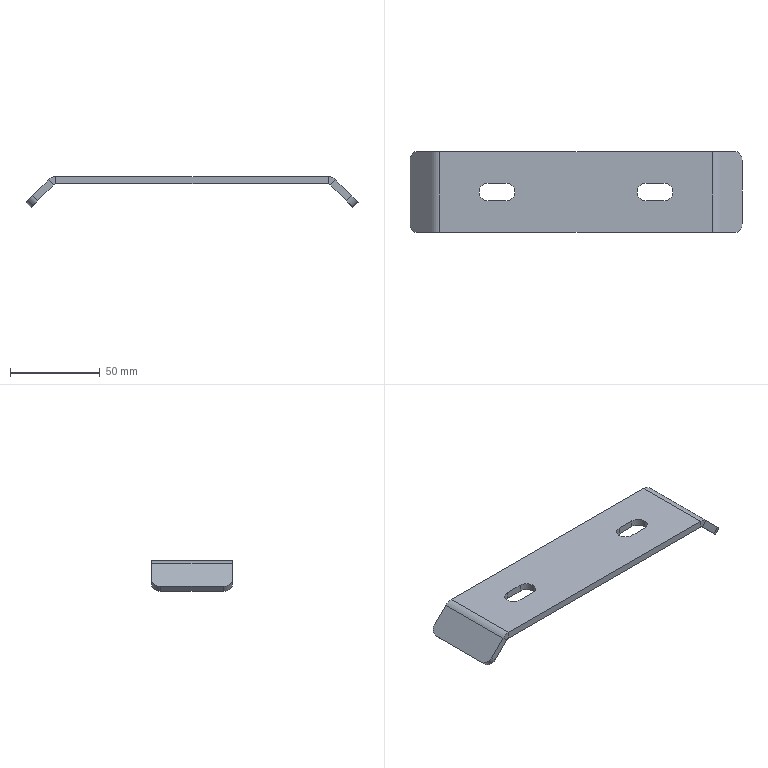Part | STEP file | PN_0071 guardrail connecting plate (spacing 140)_Default<As Machined> | 1 solid | 34 faces | box 184.912 x 45 x 17 mm | volume 33225 mm3 | plane 22 | cylinder 12 | commonest cylinder face diameters 10 x8 4 x2 12 x2